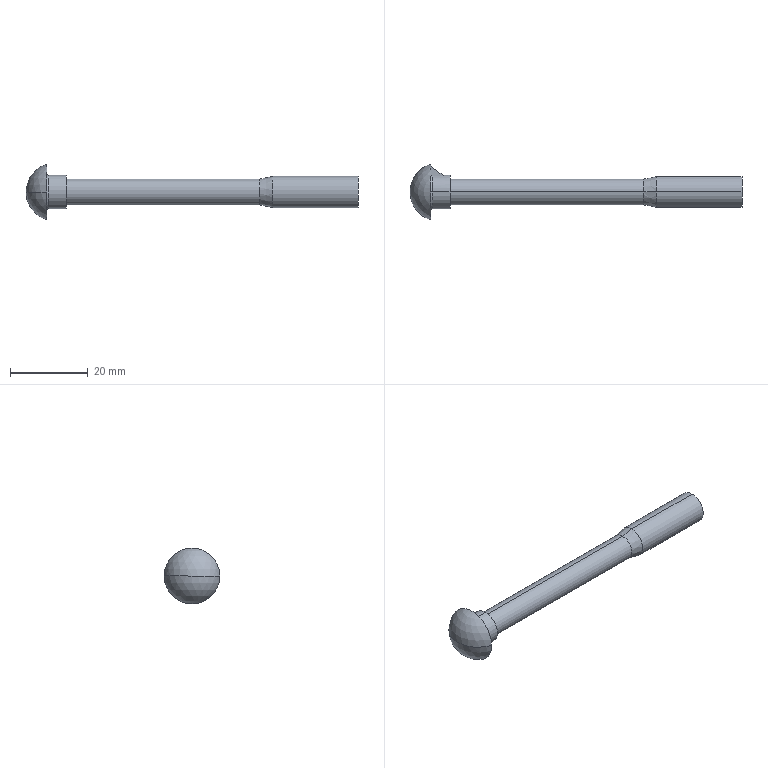Part | SolidWorks | features RevCut 2, LPattern 1, Revolution 1, Rib 1 | 1 solid | 19 faces | box 85.28 x 14.328 x 14.328 mm | volume 3773 mm3 | cylinder 6 | plane 6 | torus 3 | cone 2 | sphere 2 | commonest cylinder face diameters 6.647 x2 8 x2 8.58 x2
STEP:
#1=CARTESIAN_POINT('',(85.28,0.,4.));
#2=VERTEX_POINT('',#1);
#3=CARTESIAN_POINT('',(85.28,0.,-4.));
#4=VERTEX_POINT('',#3);
#5=CARTESIAN_POINT('',(85.28,0.,0.));
#6=DIRECTION('',(-1.,0.,0.));
#7=DIRECTION('',(0.,0.,1.));
#8=AXIS2_PLACEMENT_3D('',#5,#6,#7);
#9=CIRCLE('',#8,4.);
#10=EDGE_CURVE('',#2,#4,#9,.T.);
#11=ORIENTED_EDGE('',*,*,#10,.T.);
#12=CARTESIAN_POINT('',(63.28,0.,-4.));
#13=VERTEX_POINT('',#12);
#14=CARTESIAN_POINT('',(-31.484,0.,-4.));
#15=DIRECTION('',(-1.,0.,0.));
#16=VECTOR('',#15,1000.);
#17=LINE('',#14,#16);
#18=EDGE_CURVE('',#4,#13,#17,.T.);
#19=ORIENTED_EDGE('',*,*,#18,.T.);
#20=CARTESIAN_POINT('',(63.28,0.,4.));
#21=VERTEX_POINT('',#20);
#22=CARTESIAN_POINT('',(63.28,0.,0.));
#23=DIRECTION('',(-1.,0.,0.));
#24=DIRECTION('',(0.,0.,1.));
#25=AXIS2_PLACEMENT_3D('',#22,#23,#24);
#26=CIRCLE('',#25,4.);
#27=EDGE_CURVE('',#21,#13,#26,.T.);
#28=ORIENTED_EDGE('',*,*,#27,.F.);
#29=CARTESIAN_POINT('',(-31.484,0.,4.));
#30=DIRECTION('',(-1.,0.,0.));
#31=VECTOR('',#30,1000.);
#32=LINE('',#29,#31);
#33=EDGE_CURVE('',#2,#21,#32,.T.);
#34=ORIENTED_EDGE('',*,*,#33,.F.);
#35=EDGE_LOOP('',(#11,#19,#28,#34));
#36=FACE_OUTER_BOUND('',#35,.T.);
#37=CARTESIAN_POINT('',(-31.484,0.,0.));
#38=DIRECTION('',(-1.,0.,0.));
#39=DIRECTION('',(0.,0.,1.));
#40=AXIS2_PLACEMENT_3D('',#37,#38,#39);
#41=CYLINDRICAL_SURFACE('',#40,4.);
#42=ADVANCED_FACE('',(#36),#41,.T.);
#43=CARTESIAN_POINT('',(60.08,0.,3.324));
#44=VERTEX_POINT('',#43);
#45=CARTESIAN_POINT('',(60.08,0.,-3.323));
#46=VERTEX_POINT('',#45);
#47=CARTESIAN_POINT('',(60.08,0.,0.));
#48=DIRECTION('',(-1.,0.,0.));
#49=DIRECTION('',(0.,0.,1.));
#50=AXIS2_PLACEMENT_3D('',#47,#48,#49);
#51=CIRCLE('',#50,3.324);
#52=EDGE_CURVE('',#44,#46,#51,.T.);
#53=ORIENTED_EDGE('',*,*,#52,.F.);
#54=CARTESIAN_POINT('',(60.08,0.,3.324));
#55=DIRECTION('',(0.9784,0.,0.2068));
#56=VECTOR('',#55,1000.);
#57=LINE('',#54,#56);
#58=EDGE_CURVE('',#44,#21,#57,.T.);
#59=ORIENTED_EDGE('',*,*,#58,.T.);
#60=ORIENTED_EDGE('',*,*,#27,.T.);
#61=CARTESIAN_POINT('',(60.08,0.,-3.323));
#62=DIRECTION('',(0.9784,0.,-0.2068));
#63=VECTOR('',#62,1000.);
#64=LINE('',#61,#63);
#65=EDGE_CURVE('',#46,#13,#64,.T.);
#66=ORIENTED_EDGE('',*,*,#65,.F.);
#67=EDGE_LOOP('',(#53,#59,#60,#66));
#68=FACE_OUTER_BOUND('',#67,.T.);
#69=CARTESIAN_POINT('',(60.08,0.,0.));
#70=DIRECTION('',(1.,0.,0.));
#71=DIRECTION('',(0.,0.,-1.));
#72=AXIS2_PLACEMENT_3D('',#69,#70,#71);
#73=CONICAL_SURFACE('',#72,3.324,0.2083);
#74=ADVANCED_FACE('',(#68),#73,.T.);
#75=ORIENTED_EDGE('',*,*,#52,.T.);
#76=CARTESIAN_POINT('',(10.28,0.,-3.323));
#77=VERTEX_POINT('',#76);
#78=CARTESIAN_POINT('',(-29.816,0.,-3.324));
#79=DIRECTION('',(-1.,0.,0.));
#80=VECTOR('',#79,1000.);
#81=LINE('',#78,#80);
#82=EDGE_CURVE('',#46,#77,#81,.T.);
#83=ORIENTED_EDGE('',*,*,#82,.T.);
#84=CARTESIAN_POINT('',(10.28,0.,3.324));
#85=VERTEX_POINT('',#84);
#86=CARTESIAN_POINT('',(10.28,0.,0.));
#87=DIRECTION('',(-1.,0.,0.));
#88=DIRECTION('',(0.,0.,1.));
#89=AXIS2_PLACEMENT_3D('',#86,#87,#88);
#90=CIRCLE('',#89,3.324);
#91=EDGE_CURVE('',#85,#77,#90,.T.);
#92=ORIENTED_EDGE('',*,*,#91,.F.);
#93=CARTESIAN_POINT('',(-29.816,0.,3.324));
#94=DIRECTION('',(-1.,0.,0.));
#95=VECTOR('',#94,1000.);
#96=LINE('',#93,#95);
#97=EDGE_CURVE('',#44,#85,#96,.T.);
#98=ORIENTED_EDGE('',*,*,#97,.F.);
#99=EDGE_LOOP('',(#75,#83,#92,#98));
#100=FACE_OUTER_BOUND('',#99,.T.);
#101=CARTESIAN_POINT('',(-29.816,0.,0.));
#102=DIRECTION('',(-1.,0.,0.));
#103=DIRECTION('',(0.,0.,1.));
#104=AXIS2_PLACEMENT_3D('',#101,#102,#103);
#105=CYLINDRICAL_SURFACE('',#104,3.324);
#106=ADVANCED_FACE('',(#100),#105,.T.);
#107=CARTESIAN_POINT('',(5.28,7.164,0.));
#108=VERTEX_POINT('',#107);
#109=CARTESIAN_POINT('',(5.28,-7.164,0.));
#110=VERTEX_POINT('',#109);
#111=CARTESIAN_POINT('',(5.28,0.,0.));
#112=DIRECTION('',(-1.,0.,0.));
#113=DIRECTION('',(0.,0.,1.));
#114=AXIS2_PLACEMENT_3D('',#111,#112,#113);
#115=CIRCLE('',#114,7.164);
#116=EDGE_CURVE('',#108,#110,#115,.T.);
#117=ORIENTED_EDGE('',*,*,#116,.T.);
#118=CARTESIAN_POINT('',(0.,0.,0.));
#119=VERTEX_POINT('',#118);
#120=CARTESIAN_POINT('',(7.5,0.,0.));
#121=DIRECTION('',(0.,0.,-1.));
#122=DIRECTION('',(0.,1.,0.));
#123=AXIS2_PLACEMENT_3D('',#120,#121,#122);
#124=CIRCLE('',#123,7.5);
#125=EDGE_CURVE('',#110,#119,#124,.T.);
#126=ORIENTED_EDGE('',*,*,#125,.T.);
#127=CARTESIAN_POINT('',(7.5,0.,0.));
#128=DIRECTION('',(0.,0.,1.));
#129=DIRECTION('',(0.,-1.,0.));
#130=AXIS2_PLACEMENT_3D('',#127,#128,#129);
#131=CIRCLE('',#130,7.5);
#132=EDGE_CURVE('',#108,#119,#131,.T.);
#133=ORIENTED_EDGE('',*,*,#132,.F.);
#134=EDGE_LOOP('',(#117,#126,#133));
#135=FACE_OUTER_BOUND('',#134,.T.);
#136=CARTESIAN_POINT('',(7.5,0.,0.));
#137=DIRECTION('',(0.,0.,-1.));
#138=DIRECTION('',(0.,1.,0.));
#139=AXIS2_PLACEMENT_3D('',#136,#137,#138);
#140=SPHERICAL_SURFACE('',#139,7.5);
#141=ADVANCED_FACE('',(#135),#140,.T.);
#142=CARTESIAN_POINT('',(10.28,0.,4.29));
#143=VERTEX_POINT('',#142);
#144=CARTESIAN_POINT('',(10.28,0.,-4.29));
#145=VERTEX_POINT('',#144);
#146=CARTESIAN_POINT('',(10.28,0.,0.));
#147=DIRECTION('',(-1.,0.,0.));
#148=DIRECTION('',(0.,0.,1.));
#149=AXIS2_PLACEMENT_3D('',#146,#147,#148);
#150=CIRCLE('',#149,4.29);
#151=EDGE_CURVE('',#143,#145,#150,.T.);
#152=ORIENTED_EDGE('',*,*,#151,.T.);
#153=CARTESIAN_POINT('',(5.78,0.,-4.29));
#154=VERTEX_POINT('',#153);
#155=CARTESIAN_POINT('',(-31.484,0.,-4.29));
#156=DIRECTION('',(-1.,0.,0.));
#157=VECTOR('',#156,1000.);
#158=LINE('',#155,#157);
#159=EDGE_CURVE('',#145,#154,#158,.T.);
#160=ORIENTED_EDGE('',*,*,#159,.T.);
#161=CARTESIAN_POINT('',(5.78,4.072,-1.35));
#162=VERTEX_POINT('',#161);
#163=CARTESIAN_POINT('',(5.78,0.,0.));
#164=DIRECTION('',(-1.,0.,0.));
#165=DIRECTION('',(0.,0.,1.));
#166=AXIS2_PLACEMENT_3D('',#163,#164,#165);
#167=CIRCLE('',#166,4.29);
#168=EDGE_CURVE('',#162,#154,#167,.T.);
#169=ORIENTED_EDGE('',*,*,#168,.F.);
#170=CARTESIAN_POINT('',(8.774,4.072,-1.35));
#171=VERTEX_POINT('',#170);
#172=CARTESIAN_POINT('',(-31.484,4.072,-1.35));
#173=DIRECTION('',(-1.,0.,0.));
#174=VECTOR('',#173,1000.);
#175=LINE('',#172,#174);
#176=EDGE_CURVE('',#171,#162,#175,.T.);
#177=ORIENTED_EDGE('',*,*,#176,.F.);
#178=CARTESIAN_POINT('',(8.774,4.072,1.35));
#179=VERTEX_POINT('',#178);
#180=CARTESIAN_POINT('',(8.774,4.072,-1.35));
#181=CARTESIAN_POINT('',(8.379,4.365,-0.4658));
#182=CARTESIAN_POINT('',(8.379,4.365,0.4658));
#183=CARTESIAN_POINT('',(8.774,4.072,1.35));
#184=(BOUNDED_CURVE()B_SPLINE_CURVE(3,(#180,#181,#182,#183),.UNSPECIFIED.,.F.,.F.)B_SPLINE_CURVE_WITH_KNOTS((4,4),(5.963,6.603),.UNSPECIFIED.)CURVE()GEOMETRIC_REPRESENTATION_ITEM()RATIONAL_B_SPLINE_CURVE((1.,0.9661,0.9661,1.))REPRESENTATION_ITEM(''));
#185=EDGE_CURVE('',#171,#179,#184,.T.);
#186=ORIENTED_EDGE('',*,*,#185,.T.);
#187=CARTESIAN_POINT('',(5.78,4.072,1.35));
#188=VERTEX_POINT('',#187);
#189=CARTESIAN_POINT('',(-31.484,4.072,1.35));
#190=DIRECTION('',(-1.,0.,0.));
#191=VECTOR('',#190,1000.);
#192=LINE('',#189,#191);
#193=EDGE_CURVE('',#179,#188,#192,.T.);
#194=ORIENTED_EDGE('',*,*,#193,.T.);
#195=CARTESIAN_POINT('',(5.78,0.,4.29));
#196=VERTEX_POINT('',#195);
#197=CARTESIAN_POINT('',(5.78,0.,0.));
#198=DIRECTION('',(-1.,0.,0.));
#199=DIRECTION('',(0.,0.,1.));
#200=AXIS2_PLACEMENT_3D('',#197,#198,#199);
#201=CIRCLE('',#200,4.29);
#202=EDGE_CURVE('',#196,#188,#201,.T.);
#203=ORIENTED_EDGE('',*,*,#202,.F.);
#204=CARTESIAN_POINT('',(-31.484,0.,4.29));
#205=DIRECTION('',(-1.,0.,0.));
#206=VECTOR('',#205,1000.);
#207=LINE('',#204,#206);
#208=EDGE_CURVE('',#143,#196,#207,.T.);
#209=ORIENTED_EDGE('',*,*,#208,.F.);
#210=EDGE_LOOP('',(#152,#160,#169,#177,#186,#194,#203,#209));
#211=FACE_OUTER_BOUND('',#210,.T.);
#212=CARTESIAN_POINT('',(-31.484,0.,0.));
#213=DIRECTION('',(-1.,0.,0.));
#214=DIRECTION('',(0.,0.,1.));
#215=AXIS2_PLACEMENT_3D('',#212,#213,#214);
#216=CYLINDRICAL_SURFACE('',#215,4.29);
#217=ADVANCED_FACE('',(#211),#216,.T.);
#218=CARTESIAN_POINT('',(5.28,0.,-4.79));
#219=VERTEX_POINT('',#218);
#220=CARTESIAN_POINT('',(5.28,0.,4.79));
#221=VERTEX_POINT('',#220);
#222=CARTESIAN_POINT('',(5.28,0.,0.));
#223=DIRECTION('',(-1.,0.,0.));
#224=DIRECTION('',(0.,0.,1.));
#225=AXIS2_PLACEMENT_3D('',#222,#223,#224);
#226=CIRCLE('',#225,4.79);
#227=EDGE_CURVE('',#219,#221,#226,.T.);
#228=ORIENTED_EDGE('',*,*,#227,.F.);
#229=CARTESIAN_POINT('',(5.78,0.,-4.79));
#230=DIRECTION('',(0.,1.,0.));
#231=DIRECTION('',(0.,0.,1.));
#232=AXIS2_PLACEMENT_3D('',#229,#230,#231);
#233=CIRCLE('',#232,0.5);
#234=EDGE_CURVE('',#219,#154,#233,.T.);
#235=ORIENTED_EDGE('',*,*,#234,.T.);
#236=CARTESIAN_POINT('',(5.78,0.,0.));
#237=DIRECTION('',(-1.,0.,0.));
#238=DIRECTION('',(0.,0.,1.));
#239=AXIS2_PLACEMENT_3D('',#236,#237,#238);
#240=CIRCLE('',#239,4.29);
#241=EDGE_CURVE('',#154,#196,#240,.T.);
#242=ORIENTED_EDGE('',*,*,#241,.T.);
#243=CARTESIAN_POINT('',(5.78,0.,4.79));
#244=DIRECTION('',(0.,-1.,0.));
#245=DIRECTION('',(0.,0.,-1.));
#246=AXIS2_PLACEMENT_3D('',#243,#244,#245);
#247=CIRCLE('',#246,0.5);
#248=EDGE_CURVE('',#221,#196,#247,.T.);
#249=ORIENTED_EDGE('',*,*,#248,.F.);
#250=EDGE_LOOP('',(#228,#235,#242,#249));
#251=FACE_OUTER_BOUND('',#250,.T.);
#252=CARTESIAN_POINT('',(5.78,0.,0.));
#253=DIRECTION('',(-1.,0.,0.));
#254=DIRECTION('',(0.,0.,1.));
#255=AXIS2_PLACEMENT_3D('',#252,#253,#254);
#256=TOROIDAL_SURFACE('',#255,4.79,0.5);
#257=ADVANCED_FACE('',(#251),#256,.F.);
#258=CARTESIAN_POINT('',(5.28,4.596,1.35));
#259=VERTEX_POINT('',#258);
#260=CARTESIAN_POINT('',(5.28,0.,0.));
#261=DIRECTION('',(-1.,0.,0.));
#262=DIRECTION('',(0.,0.,1.));
#263=AXIS2_PLACEMENT_3D('',#260,#261,#262);
#264=CIRCLE('',#263,4.79);
#265=EDGE_CURVE('',#221,#259,#264,.T.);
#266=ORIENTED_EDGE('',*,*,#265,.F.);
#267=ORIENTED_EDGE('',*,*,#248,.T.);
#268=ORIENTED_EDGE('',*,*,#202,.T.);
#269=CARTESIAN_POINT('',(5.78,4.072,1.35));
#270=CARTESIAN_POINT('',(5.647,4.072,1.35));
#271=CARTESIAN_POINT('',(5.513,4.133,1.35));
#272=CARTESIAN_POINT('',(5.331,4.328,1.35));
#273=CARTESIAN_POINT('',(5.28,4.463,1.35));
#274=CARTESIAN_POINT('',(5.28,4.596,1.35));
#275=B_SPLINE_CURVE_WITH_KNOTS('',3,(#269,#270,#271,#272,#273,#274),.UNSPECIFIED.,.F.,.F.,(4,2,4),(0.002846,0.003245,0.003645),.UNSPECIFIED.);
#276=EDGE_CURVE('',#188,#259,#275,.T.);
#277=ORIENTED_EDGE('',*,*,#276,.T.);
#278=EDGE_LOOP('',(#266,#267,#268,#277));
#279=FACE_OUTER_BOUND('',#278,.T.);
#280=CARTESIAN_POINT('',(5.78,0.,0.));
#281=DIRECTION('',(-1.,0.,0.));
#282=DIRECTION('',(0.,0.,1.));
#283=AXIS2_PLACEMENT_3D('',#280,#281,#282);
#284=TOROIDAL_SURFACE('',#283,4.79,0.5);
#285=ADVANCED_FACE('',(#279),#284,.F.);
#286=ORIENTED_EDGE('',*,*,#234,.F.);
#287=CARTESIAN_POINT('',(5.28,4.596,-1.35));
#288=VERTEX_POINT('',#287);
#289=CARTESIAN_POINT('',(5.28,0.,0.));
#290=DIRECTION('',(-1.,0.,0.));
#291=DIRECTION('',(0.,0.,1.));
#292=AXIS2_PLACEMENT_3D('',#289,#290,#291);
#293=CIRCLE('',#292,4.79);
#294=EDGE_CURVE('',#288,#219,#293,.T.);
#295=ORIENTED_EDGE('',*,*,#294,.F.);
#296=CARTESIAN_POINT('',(5.78,4.072,-1.35));
#297=CARTESIAN_POINT('',(5.647,4.072,-1.35));
#298=CARTESIAN_POINT('',(5.513,4.133,-1.35));
#299=CARTESIAN_POINT('',(5.331,4.328,-1.35));
#300=CARTESIAN_POINT('',(5.28,4.463,-1.35));
#301=CARTESIAN_POINT('',(5.28,4.596,-1.35));
#302=B_SPLINE_CURVE_WITH_KNOTS('',3,(#296,#297,#298,#299,#300,#301),.UNSPECIFIED.,.F.,.F.,(4,2,4),(0.002846,0.003245,0.003645),.UNSPECIFIED.);
#303=EDGE_CURVE('',#162,#288,#302,.T.);
#304=ORIENTED_EDGE('',*,*,#303,.F.);
#305=ORIENTED_EDGE('',*,*,#168,.T.);
#306=EDGE_LOOP('',(#286,#295,#304,#305));
#307=FACE_OUTER_BOUND('',#306,.T.);
#308=CARTESIAN_POINT('',(5.78,0.,0.));
#309=DIRECTION('',(-1.,0.,0.));
#310=DIRECTION('',(0.,0.,1.));
#311=AXIS2_PLACEMENT_3D('',#308,#309,#310);
#312=TOROIDAL_SURFACE('',#311,4.79,0.5);
#313=ADVANCED_FACE('',(#307),#312,.F.);
#314=ORIENTED_EDGE('',*,*,#159,.F.);
#315=CARTESIAN_POINT('',(10.28,0.,0.));
#316=DIRECTION('',(-1.,0.,0.));
#317=DIRECTION('',(0.,0.,1.));
#318=AXIS2_PLACEMENT_3D('',#315,#316,#317);
#319=CIRCLE('',#318,4.29);
#320=EDGE_CURVE('',#145,#143,#319,.T.);
#321=ORIENTED_EDGE('',*,*,#320,.T.);
#322=ORIENTED_EDGE('',*,*,#208,.T.);
#323=ORIENTED_EDGE('',*,*,#241,.F.);
#324=EDGE_LOOP('',(#314,#321,#322,#323));
#325=FACE_OUTER_BOUND('',#324,.T.);
#326=CARTESIAN_POINT('',(-31.484,0.,0.));
#327=DIRECTION('',(-1.,0.,0.));
#328=DIRECTION('',(0.,0.,1.));
#329=AXIS2_PLACEMENT_3D('',#326,#327,#328);
#330=CYLINDRICAL_SURFACE('',#329,4.29);
#331=ADVANCED_FACE('',(#325),#330,.T.);
#332=ORIENTED_EDGE('',*,*,#151,.F.);
#333=ORIENTED_EDGE('',*,*,#320,.F.);
#334=EDGE_LOOP('',(#332,#333));
#335=FACE_OUTER_BOUND('',#334,.T.);
#336=ORIENTED_EDGE('',*,*,#91,.T.);
#337=CARTESIAN_POINT('',(10.28,0.,0.));
#338=DIRECTION('',(-1.,0.,0.));
#339=DIRECTION('',(0.,0.,1.));
#340=AXIS2_PLACEMENT_3D('',#337,#338,#339);
#341=CIRCLE('',#340,3.324);
#342=EDGE_CURVE('',#77,#85,#341,.T.);
#343=ORIENTED_EDGE('',*,*,#342,.T.);
#344=EDGE_LOOP('',(#336,#343));
#345=FACE_BOUND('',#344,.T.);
#346=CARTESIAN_POINT('',(10.28,4.,0.));
#347=DIRECTION('',(-1.,0.,0.));
#348=DIRECTION('',(0.,0.,1.));
#349=AXIS2_PLACEMENT_3D('',#346,#347,#348);
#350=PLANE('',#349);
#351=ADVANCED_FACE('',(#335,#345),#350,.F.);
#352=ORIENTED_EDGE('',*,*,#125,.F.);
#353=CARTESIAN_POINT('',(5.28,0.,0.));
#354=DIRECTION('',(-1.,0.,0.));
#355=DIRECTION('',(0.,0.,1.));
#356=AXIS2_PLACEMENT_3D('',#353,#354,#355);
#357=CIRCLE('',#356,7.164);
#358=EDGE_CURVE('',#110,#108,#357,.T.);
#359=ORIENTED_EDGE('',*,*,#358,.T.);
#360=ORIENTED_EDGE('',*,*,#132,.T.);
#361=EDGE_LOOP('',(#352,#359,#360));
#362=FACE_OUTER_BOUND('',#361,.T.);
#363=CARTESIAN_POINT('',(7.5,0.,0.));
#364=DIRECTION('',(0.,0.,-1.));
#365=DIRECTION('',(0.,1.,0.));
#366=AXIS2_PLACEMENT_3D('',#363,#364,#365);
#367=SPHERICAL_SURFACE('',#366,7.5);
#368=ADVANCED_FACE('',(#362),#367,.T.);
#369=ORIENTED_EDGE('',*,*,#294,.T.);
#370=ORIENTED_EDGE('',*,*,#227,.T.);
#371=ORIENTED_EDGE('',*,*,#265,.T.);
#372=CARTESIAN_POINT('',(5.28,6.664,1.35));
#373=VERTEX_POINT('',#372);
#374=CARTESIAN_POINT('',(5.28,4.79,1.35));
#375=DIRECTION('',(0.,1.,0.));
#376=VECTOR('',#375,1000.);
#377=LINE('',#374,#376);
#378=EDGE_CURVE('',#259,#373,#377,.T.);
#379=ORIENTED_EDGE('',*,*,#378,.T.);
#380=CARTESIAN_POINT('',(5.28,6.664,-1.35));
#381=VERTEX_POINT('',#380);
#382=CARTESIAN_POINT('',(5.28,6.664,0.));
#383=DIRECTION('',(0.,0.,-1.));
#384=VECTOR('',#383,1000.);
#385=LINE('',#382,#384);
#386=EDGE_CURVE('',#373,#381,#385,.T.);
#387=ORIENTED_EDGE('',*,*,#386,.T.);
#388=CARTESIAN_POINT('',(5.28,4.79,-1.35));
#389=DIRECTION('',(0.,1.,0.));
#390=VECTOR('',#389,1000.);
#391=LINE('',#388,#390);
#392=EDGE_CURVE('',#288,#381,#391,.T.);
#393=ORIENTED_EDGE('',*,*,#392,.F.);
#394=EDGE_LOOP('',(#369,#370,#371,#379,#387,#393));
#395=FACE_BOUND('',#394,.T.);
#396=ORIENTED_EDGE('',*,*,#116,.F.);
#397=ORIENTED_EDGE('',*,*,#358,.F.);
#398=EDGE_LOOP('',(#396,#397));
#399=FACE_OUTER_BOUND('',#398,.T.);
#400=CARTESIAN_POINT('',(5.28,4.79,0.));
#401=DIRECTION('',(-1.,0.,0.));
#402=DIRECTION('',(0.,0.,1.));
#403=AXIS2_PLACEMENT_3D('',#400,#401,#402);
#404=PLANE('',#403);
#405=ADVANCED_FACE('',(#395,#399),#404,.F.);
#406=ORIENTED_EDGE('',*,*,#185,.F.);
#407=CARTESIAN_POINT('',(8.48,4.29,-1.35));
#408=DIRECTION('',(-0.8031,0.5958,0.));
#409=VECTOR('',#408,1000.);
#410=LINE('',#407,#409);
#411=EDGE_CURVE('',#171,#381,#410,.T.);
#412=ORIENTED_EDGE('',*,*,#411,.T.);
#413=ORIENTED_EDGE('',*,*,#386,.F.);
#414=CARTESIAN_POINT('',(8.48,4.29,1.35));
#415=DIRECTION('',(-0.8031,0.5958,0.));
#416=VECTOR('',#415,1000.);
#417=LINE('',#414,#416);
#418=EDGE_CURVE('',#179,#373,#417,.T.);
#419=ORIENTED_EDGE('',*,*,#418,.F.);
#420=EDGE_LOOP('',(#406,#412,#413,#419));
#421=FACE_OUTER_BOUND('',#420,.T.);
#422=CARTESIAN_POINT('',(8.48,4.29,0.));
#423=DIRECTION('',(0.5958,0.8031,0.));
#424=DIRECTION('',(-0.8031,0.5958,0.));
#425=AXIS2_PLACEMENT_3D('',#422,#423,#424);
#426=PLANE('',#425);
#427=ADVANCED_FACE('',(#421),#426,.T.);
#428=ORIENTED_EDGE('',*,*,#276,.F.);
#429=ORIENTED_EDGE('',*,*,#193,.F.);
#430=ORIENTED_EDGE('',*,*,#418,.T.);
#431=ORIENTED_EDGE('',*,*,#378,.F.);
#432=EDGE_LOOP('',(#428,#429,#430,#431));
#433=FACE_OUTER_BOUND('',#432,.T.);
#434=CARTESIAN_POINT('',(42.64,0.,1.35));
#435=DIRECTION('',(0.,0.,1.));
#436=DIRECTION('',(1.,0.,0.));
#437=AXIS2_PLACEMENT_3D('',#434,#435,#436);
#438=PLANE('',#437);
#439=ADVANCED_FACE('',(#433),#438,.T.);
#440=ORIENTED_EDGE('',*,*,#411,.F.);
#441=ORIENTED_EDGE('',*,*,#176,.T.);
#442=ORIENTED_EDGE('',*,*,#303,.T.);
#443=ORIENTED_EDGE('',*,*,#392,.T.);
#444=EDGE_LOOP('',(#440,#441,#442,#443));
#445=FACE_OUTER_BOUND('',#444,.T.);
#446=CARTESIAN_POINT('',(42.64,0.,-1.35));
#447=DIRECTION('',(0.,0.,1.));
#448=DIRECTION('',(1.,0.,0.));
#449=AXIS2_PLACEMENT_3D('',#446,#447,#448);
#450=PLANE('',#449);
#451=ADVANCED_FACE('',(#445),#450,.F.);
#452=ORIENTED_EDGE('',*,*,#82,.F.);
#453=CARTESIAN_POINT('',(60.08,0.,0.));
#454=DIRECTION('',(-1.,0.,0.));
#455=DIRECTION('',(0.,0.,1.));
#456=AXIS2_PLACEMENT_3D('',#453,#454,#455);
#457=CIRCLE('',#456,3.324);
#458=EDGE_CURVE('',#46,#44,#457,.T.);
#459=ORIENTED_EDGE('',*,*,#458,.T.);
#460=ORIENTED_EDGE('',*,*,#97,.T.);
#461=ORIENTED_EDGE('',*,*,#342,.F.);
#462=EDGE_LOOP('',(#452,#459,#460,#461));
#463=FACE_OUTER_BOUND('',#462,.T.);
#464=CARTESIAN_POINT('',(-29.816,0.,0.));
#465=DIRECTION('',(-1.,0.,0.));
#466=DIRECTION('',(0.,0.,1.));
#467=AXIS2_PLACEMENT_3D('',#464,#465,#466);
#468=CYLINDRICAL_SURFACE('',#467,3.324);
#469=ADVANCED_FACE('',(#463),#468,.T.);
#470=ORIENTED_EDGE('',*,*,#58,.F.);
#471=ORIENTED_EDGE('',*,*,#458,.F.);
#472=ORIENTED_EDGE('',*,*,#65,.T.);
#473=CARTESIAN_POINT('',(63.28,0.,0.));
#474=DIRECTION('',(-1.,0.,0.));
#475=DIRECTION('',(0.,0.,1.));
#476=AXIS2_PLACEMENT_3D('',#473,#474,#475);
#477=CIRCLE('',#476,4.);
#478=EDGE_CURVE('',#13,#21,#477,.T.);
#479=ORIENTED_EDGE('',*,*,#478,.T.);
#480=EDGE_LOOP('',(#470,#471,#472,#479));
#481=FACE_OUTER_BOUND('',#480,.T.);
#482=CARTESIAN_POINT('',(60.08,0.,0.));
#483=DIRECTION('',(1.,0.,0.));
#484=DIRECTION('',(0.,0.,-1.));
#485=AXIS2_PLACEMENT_3D('',#482,#483,#484);
#486=CONICAL_SURFACE('',#485,3.324,0.2083);
#487=ADVANCED_FACE('',(#481),#486,.T.);
#488=ORIENTED_EDGE('',*,*,#10,.F.);
#489=CARTESIAN_POINT('',(85.28,0.,0.));
#490=DIRECTION('',(-1.,0.,0.));
#491=DIRECTION('',(0.,0.,1.));
#492=AXIS2_PLACEMENT_3D('',#489,#490,#491);
#493=CIRCLE('',#492,4.);
#494=EDGE_CURVE('',#4,#2,#493,.T.);
#495=ORIENTED_EDGE('',*,*,#494,.F.);
#496=EDGE_LOOP('',(#488,#495));
#497=FACE_OUTER_BOUND('',#496,.T.);
#498=CARTESIAN_POINT('',(85.28,0.,0.));
#499=DIRECTION('',(-1.,0.,0.));
#500=DIRECTION('',(0.,0.,1.));
#501=AXIS2_PLACEMENT_3D('',#498,#499,#500);
#502=PLANE('',#501);
#503=ADVANCED_FACE('',(#497),#502,.F.);
#504=ORIENTED_EDGE('',*,*,#18,.F.);
#505=ORIENTED_EDGE('',*,*,#494,.T.);
#506=ORIENTED_EDGE('',*,*,#33,.T.);
#507=ORIENTED_EDGE('',*,*,#478,.F.);
#508=EDGE_LOOP('',(#504,#505,#506,#507));
#509=FACE_OUTER_BOUND('',#508,.T.);
#510=CARTESIAN_POINT('',(-31.484,0.,0.));
#511=DIRECTION('',(-1.,0.,0.));
#512=DIRECTION('',(0.,0.,1.));
#513=AXIS2_PLACEMENT_3D('',#510,#511,#512);
#514=CYLINDRICAL_SURFACE('',#513,4.);
#515=ADVANCED_FACE('',(#509),#514,.T.);
#516=CLOSED_SHELL('',(#42,#74,#106,#141,#217,#257,#285,#313,#331,#351,#368,#405,#427,#439,#451,#469,#487,#503,#515));
#517=MANIFOLD_SOLID_BREP('',#516);
#518=CARTESIAN_POINT('',(0.,0.,0.));
#519=DIRECTION('',(0.,0.,1.));
#520=DIRECTION('',(1.,0.,0.));
#521=AXIS2_PLACEMENT_3D('',#518,#519,#520);
#522=(LENGTH_UNIT()NAMED_UNIT(*)SI_UNIT(.MILLI.,.METRE.));
#523=UNCERTAINTY_MEASURE_WITH_UNIT(LENGTH_MEASURE(0.00001),#522,'','');
#524=(NAMED_UNIT(*)PLANE_ANGLE_UNIT()SI_UNIT($,.RADIAN.));
#525=(NAMED_UNIT(*)SI_UNIT($,.STERADIAN.)SOLID_ANGLE_UNIT());
#526=(GEOMETRIC_REPRESENTATION_CONTEXT(3)GLOBAL_UNCERTAINTY_ASSIGNED_CONTEXT((#523))GLOBAL_UNIT_ASSIGNED_CONTEXT((#522,#524,#525))REPRESENTATION_CONTEXT('',''));
#527=ADVANCED_BREP_SHAPE_REPRESENTATION('',(#517,#521),#526);